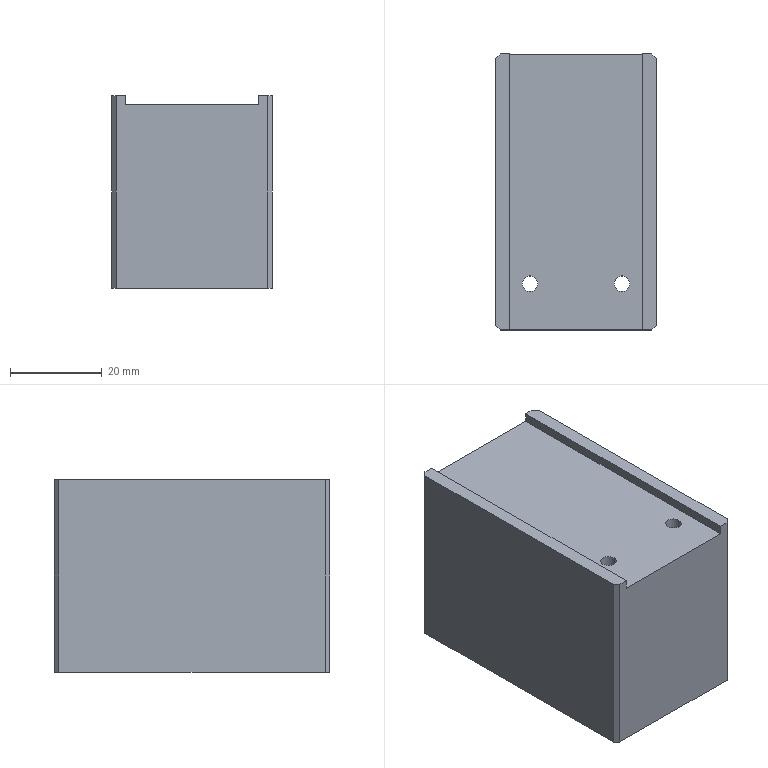Part | STEP file | PN_0025 | 1 solid | 40 faces | box 35 x 60 x 42 mm | volume 82188 mm3 | cylinder 16 | plane 16 | cone 8 | commonest cylinder face diameters 3.4 x4 4 x4 4.2 x4 6.5 x4